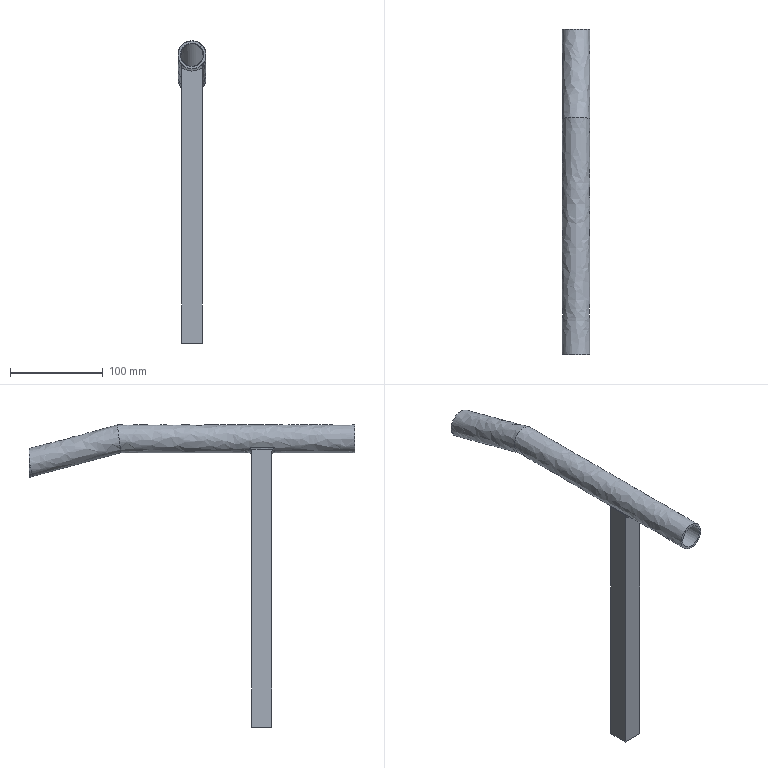Part | NX | features solid 2 | 1 solid | 22 faces | box 30 x 350.001 x 325 mm | volume 130270 mm3 | plane 11 | spline 10 | cylinder 1 | commonest cylinder face diameters 30 x1